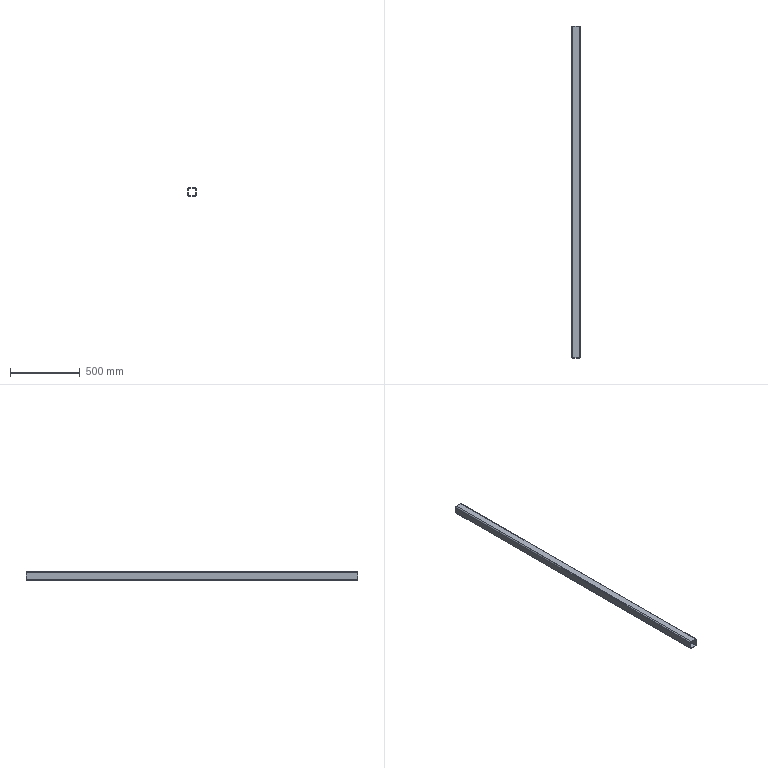Part | SolidWorks | features BaseBody 1 | 1 solid | 18 faces | box 60 x 2380 x 60 mm | volume 2034416 mm3 | plane 10 | cylinder 8 | commonest cylinder face diameters 8 x4 16 x4
STEP:
#1=CARTESIAN_POINT('',(696.,2432.,-1248.));
#2=VERTEX_POINT('',#1);
#3=CARTESIAN_POINT('',(696.,2432.,-1292.));
#4=VERTEX_POINT('',#3);
#5=CARTESIAN_POINT('',(696.,2432.,-1292.));
#6=DIRECTION('',(0.,0.,-1.));
#7=VECTOR('',#6,1000.);
#8=LINE('',#5,#7);
#9=EDGE_CURVE('',#2,#4,#8,.T.);
#10=ORIENTED_EDGE('',*,*,#9,.T.);
#11=CARTESIAN_POINT('',(696.,52.,-1292.));
#12=VERTEX_POINT('',#11);
#13=CARTESIAN_POINT('',(696.,2462.,-1292.));
#14=DIRECTION('',(0.,-1.,0.));
#15=VECTOR('',#14,1000.);
#16=LINE('',#13,#15);
#17=EDGE_CURVE('',#4,#12,#16,.T.);
#18=ORIENTED_EDGE('',*,*,#17,.T.);
#19=CARTESIAN_POINT('',(696.,52.,-1248.));
#20=VERTEX_POINT('',#19);
#21=CARTESIAN_POINT('',(696.,52.,-1292.));
#22=DIRECTION('',(0.,0.,1.));
#23=VECTOR('',#22,1000.);
#24=LINE('',#21,#23);
#25=EDGE_CURVE('',#12,#20,#24,.T.);
#26=ORIENTED_EDGE('',*,*,#25,.T.);
#27=CARTESIAN_POINT('',(696.,2462.,-1248.));
#28=DIRECTION('',(0.,1.,0.));
#29=VECTOR('',#28,1000.);
#30=LINE('',#27,#29);
#31=EDGE_CURVE('',#20,#2,#30,.T.);
#32=ORIENTED_EDGE('',*,*,#31,.T.);
#33=EDGE_LOOP('',(#10,#18,#26,#32));
#34=FACE_OUTER_BOUND('',#33,.T.);
#35=CARTESIAN_POINT('',(696.,2462.,-1292.));
#36=DIRECTION('',(-1.,0.,0.));
#37=DIRECTION('',(0.,0.,1.));
#38=AXIS2_PLACEMENT_3D('',#35,#36,#37);
#39=PLANE('',#38);
#40=ADVANCED_FACE('',(#34),#39,.T.);
#41=ORIENTED_EDGE('',*,*,#17,.F.);
#42=CARTESIAN_POINT('',(692.,2432.,-1296.));
#43=VERTEX_POINT('',#42);
#44=CARTESIAN_POINT('',(692.,2432.,-1292.));
#45=DIRECTION('',(0.,-1.,0.));
#46=DIRECTION('',(0.,0.,-1.));
#47=AXIS2_PLACEMENT_3D('',#44,#45,#46);
#48=CIRCLE('',#47,4.);
#49=EDGE_CURVE('',#43,#4,#48,.T.);
#50=ORIENTED_EDGE('',*,*,#49,.F.);
#51=CARTESIAN_POINT('',(692.,52.,-1296.));
#52=VERTEX_POINT('',#51);
#53=CARTESIAN_POINT('',(692.,2462.,-1296.));
#54=DIRECTION('',(0.,1.,0.));
#55=VECTOR('',#54,1000.);
#56=LINE('',#53,#55);
#57=EDGE_CURVE('',#52,#43,#56,.T.);
#58=ORIENTED_EDGE('',*,*,#57,.F.);
#59=CARTESIAN_POINT('',(692.,52.,-1292.));
#60=DIRECTION('',(0.,1.,0.));
#61=DIRECTION('',(0.,0.,-1.));
#62=AXIS2_PLACEMENT_3D('',#59,#60,#61);
#63=CIRCLE('',#62,4.);
#64=EDGE_CURVE('',#12,#52,#63,.T.);
#65=ORIENTED_EDGE('',*,*,#64,.F.);
#66=EDGE_LOOP('',(#41,#50,#58,#65));
#67=FACE_OUTER_BOUND('',#66,.T.);
#68=CARTESIAN_POINT('',(692.,2462.,-1292.));
#69=DIRECTION('',(0.,-1.,0.));
#70=DIRECTION('',(0.,0.,-1.));
#71=AXIS2_PLACEMENT_3D('',#68,#69,#70);
#72=CYLINDRICAL_SURFACE('',#71,4.);
#73=ADVANCED_FACE('',(#67),#72,.F.);
#74=CARTESIAN_POINT('',(692.,2432.,-1244.));
#75=VERTEX_POINT('',#74);
#76=CARTESIAN_POINT('',(692.,2432.,-1248.));
#77=DIRECTION('',(0.,-1.,0.));
#78=DIRECTION('',(0.,0.,-1.));
#79=AXIS2_PLACEMENT_3D('',#76,#77,#78);
#80=CIRCLE('',#79,4.);
#81=EDGE_CURVE('',#2,#75,#80,.T.);
#82=ORIENTED_EDGE('',*,*,#81,.T.);
#83=CARTESIAN_POINT('',(648.,2432.,-1244.));
#84=VERTEX_POINT('',#83);
#85=CARTESIAN_POINT('',(25.,2432.,-1244.));
#86=DIRECTION('',(-1.,0.,0.));
#87=VECTOR('',#86,1000.);
#88=LINE('',#85,#87);
#89=EDGE_CURVE('',#75,#84,#88,.T.);
#90=ORIENTED_EDGE('',*,*,#89,.T.);
#91=CARTESIAN_POINT('',(644.,2432.,-1248.));
#92=VERTEX_POINT('',#91);
#93=CARTESIAN_POINT('',(648.,2432.,-1248.));
#94=DIRECTION('',(0.,-1.,0.));
#95=DIRECTION('',(0.,0.,-1.));
#96=AXIS2_PLACEMENT_3D('',#93,#94,#95);
#97=CIRCLE('',#96,4.);
#98=EDGE_CURVE('',#84,#92,#97,.T.);
#99=ORIENTED_EDGE('',*,*,#98,.T.);
#100=CARTESIAN_POINT('',(644.,2432.,-1292.));
#101=VERTEX_POINT('',#100);
#102=CARTESIAN_POINT('',(644.,2432.,-1248.));
#103=DIRECTION('',(0.,0.,-1.));
#104=VECTOR('',#103,1000.);
#105=LINE('',#102,#104);
#106=EDGE_CURVE('',#92,#101,#105,.T.);
#107=ORIENTED_EDGE('',*,*,#106,.T.);
#108=CARTESIAN_POINT('',(648.,2432.,-1296.));
#109=VERTEX_POINT('',#108);
#110=CARTESIAN_POINT('',(648.,2432.,-1292.));
#111=DIRECTION('',(0.,-1.,0.));
#112=DIRECTION('',(0.,0.,-1.));
#113=AXIS2_PLACEMENT_3D('',#110,#111,#112);
#114=CIRCLE('',#113,4.);
#115=EDGE_CURVE('',#101,#109,#114,.T.);
#116=ORIENTED_EDGE('',*,*,#115,.T.);
#117=CARTESIAN_POINT('',(25.,2432.,-1296.));
#118=DIRECTION('',(1.,0.,0.));
#119=VECTOR('',#118,1000.);
#120=LINE('',#117,#119);
#121=EDGE_CURVE('',#109,#43,#120,.T.);
#122=ORIENTED_EDGE('',*,*,#121,.T.);
#123=ORIENTED_EDGE('',*,*,#49,.T.);
#124=ORIENTED_EDGE('',*,*,#9,.F.);
#125=EDGE_LOOP('',(#82,#90,#99,#107,#116,#122,#123,#124));
#126=FACE_BOUND('',#125,.T.);
#127=CARTESIAN_POINT('',(648.,2432.,-1240.));
#128=VERTEX_POINT('',#127);
#129=CARTESIAN_POINT('',(692.,2432.,-1240.));
#130=VERTEX_POINT('',#129);
#131=CARTESIAN_POINT('',(25.,2432.,-1240.));
#132=DIRECTION('',(1.,0.,0.));
#133=VECTOR('',#132,1000.);
#134=LINE('',#131,#133);
#135=EDGE_CURVE('',#128,#130,#134,.T.);
#136=ORIENTED_EDGE('',*,*,#135,.T.);
#137=CARTESIAN_POINT('',(700.,2432.,-1248.));
#138=VERTEX_POINT('',#137);
#139=CARTESIAN_POINT('',(692.,2432.,-1248.));
#140=DIRECTION('',(0.,1.,0.));
#141=DIRECTION('',(0.,0.,-1.));
#142=AXIS2_PLACEMENT_3D('',#139,#140,#141);
#143=CIRCLE('',#142,8.);
#144=EDGE_CURVE('',#130,#138,#143,.T.);
#145=ORIENTED_EDGE('',*,*,#144,.T.);
#146=CARTESIAN_POINT('',(700.,2432.,-1292.));
#147=VERTEX_POINT('',#146);
#148=CARTESIAN_POINT('',(700.,2432.,-1248.));
#149=DIRECTION('',(0.,0.,-1.));
#150=VECTOR('',#149,1000.);
#151=LINE('',#148,#150);
#152=EDGE_CURVE('',#138,#147,#151,.T.);
#153=ORIENTED_EDGE('',*,*,#152,.T.);
#154=CARTESIAN_POINT('',(692.,2432.,-1300.));
#155=VERTEX_POINT('',#154);
#156=CARTESIAN_POINT('',(692.,2432.,-1292.));
#157=DIRECTION('',(0.,1.,0.));
#158=DIRECTION('',(0.,0.,-1.));
#159=AXIS2_PLACEMENT_3D('',#156,#157,#158);
#160=CIRCLE('',#159,8.);
#161=EDGE_CURVE('',#147,#155,#160,.T.);
#162=ORIENTED_EDGE('',*,*,#161,.T.);
#163=CARTESIAN_POINT('',(648.,2432.,-1300.));
#164=VERTEX_POINT('',#163);
#165=CARTESIAN_POINT('',(25.,2432.,-1300.));
#166=DIRECTION('',(-1.,0.,0.));
#167=VECTOR('',#166,1000.);
#168=LINE('',#165,#167);
#169=EDGE_CURVE('',#155,#164,#168,.T.);
#170=ORIENTED_EDGE('',*,*,#169,.T.);
#171=CARTESIAN_POINT('',(640.,2432.,-1292.));
#172=VERTEX_POINT('',#171);
#173=CARTESIAN_POINT('',(648.,2432.,-1292.));
#174=DIRECTION('',(0.,1.,0.));
#175=DIRECTION('',(0.,0.,-1.));
#176=AXIS2_PLACEMENT_3D('',#173,#174,#175);
#177=CIRCLE('',#176,8.);
#178=EDGE_CURVE('',#164,#172,#177,.T.);
#179=ORIENTED_EDGE('',*,*,#178,.T.);
#180=CARTESIAN_POINT('',(640.,2432.,-1248.));
#181=VERTEX_POINT('',#180);
#182=CARTESIAN_POINT('',(640.,2432.,-1248.));
#183=DIRECTION('',(0.,0.,1.));
#184=VECTOR('',#183,1000.);
#185=LINE('',#182,#184);
#186=EDGE_CURVE('',#172,#181,#185,.T.);
#187=ORIENTED_EDGE('',*,*,#186,.T.);
#188=CARTESIAN_POINT('',(648.,2432.,-1248.));
#189=DIRECTION('',(0.,1.,0.));
#190=DIRECTION('',(0.,0.,-1.));
#191=AXIS2_PLACEMENT_3D('',#188,#189,#190);
#192=CIRCLE('',#191,8.);
#193=EDGE_CURVE('',#181,#128,#192,.T.);
#194=ORIENTED_EDGE('',*,*,#193,.T.);
#195=EDGE_LOOP('',(#136,#145,#153,#162,#170,#179,#187,#194));
#196=FACE_OUTER_BOUND('',#195,.T.);
#197=CARTESIAN_POINT('',(25.,2432.,-1248.));
#198=DIRECTION('',(0.,1.,0.));
#199=DIRECTION('',(0.,0.,1.));
#200=AXIS2_PLACEMENT_3D('',#197,#198,#199);
#201=PLANE('',#200);
#202=ADVANCED_FACE('',(#126,#196),#201,.T.);
#203=CARTESIAN_POINT('',(692.,52.,-1244.));
#204=VERTEX_POINT('',#203);
#205=CARTESIAN_POINT('',(692.,2462.,-1244.));
#206=DIRECTION('',(0.,-1.,0.));
#207=VECTOR('',#206,1000.);
#208=LINE('',#205,#207);
#209=EDGE_CURVE('',#75,#204,#208,.T.);
#210=ORIENTED_EDGE('',*,*,#209,.F.);
#211=ORIENTED_EDGE('',*,*,#81,.F.);
#212=ORIENTED_EDGE('',*,*,#31,.F.);
#213=CARTESIAN_POINT('',(692.,52.,-1248.));
#214=DIRECTION('',(0.,1.,0.));
#215=DIRECTION('',(0.,0.,-1.));
#216=AXIS2_PLACEMENT_3D('',#213,#214,#215);
#217=CIRCLE('',#216,4.);
#218=EDGE_CURVE('',#204,#20,#217,.T.);
#219=ORIENTED_EDGE('',*,*,#218,.F.);
#220=EDGE_LOOP('',(#210,#211,#212,#219));
#221=FACE_OUTER_BOUND('',#220,.T.);
#222=CARTESIAN_POINT('',(692.,2462.,-1248.));
#223=DIRECTION('',(0.,-1.,0.));
#224=DIRECTION('',(0.,0.,-1.));
#225=AXIS2_PLACEMENT_3D('',#222,#223,#224);
#226=CYLINDRICAL_SURFACE('',#225,4.);
#227=ADVANCED_FACE('',(#221),#226,.F.);
#228=ORIENTED_EDGE('',*,*,#218,.T.);
#229=ORIENTED_EDGE('',*,*,#25,.F.);
#230=ORIENTED_EDGE('',*,*,#64,.T.);
#231=CARTESIAN_POINT('',(648.,52.,-1296.));
#232=VERTEX_POINT('',#231);
#233=CARTESIAN_POINT('',(648.,52.,-1296.));
#234=DIRECTION('',(-1.,0.,0.));
#235=VECTOR('',#234,1000.);
#236=LINE('',#233,#235);
#237=EDGE_CURVE('',#52,#232,#236,.T.);
#238=ORIENTED_EDGE('',*,*,#237,.T.);
#239=CARTESIAN_POINT('',(644.,52.,-1292.));
#240=VERTEX_POINT('',#239);
#241=CARTESIAN_POINT('',(648.,52.,-1292.));
#242=DIRECTION('',(0.,1.,0.));
#243=DIRECTION('',(0.,0.,-1.));
#244=AXIS2_PLACEMENT_3D('',#241,#242,#243);
#245=CIRCLE('',#244,4.);
#246=EDGE_CURVE('',#232,#240,#245,.T.);
#247=ORIENTED_EDGE('',*,*,#246,.T.);
#248=CARTESIAN_POINT('',(644.,52.,-1248.));
#249=VERTEX_POINT('',#248);
#250=CARTESIAN_POINT('',(644.,52.,530.));
#251=DIRECTION('',(0.,0.,1.));
#252=VECTOR('',#251,1000.);
#253=LINE('',#250,#252);
#254=EDGE_CURVE('',#240,#249,#253,.T.);
#255=ORIENTED_EDGE('',*,*,#254,.T.);
#256=CARTESIAN_POINT('',(648.,52.,-1244.));
#257=VERTEX_POINT('',#256);
#258=CARTESIAN_POINT('',(648.,52.,-1248.));
#259=DIRECTION('',(0.,1.,0.));
#260=DIRECTION('',(0.,0.,-1.));
#261=AXIS2_PLACEMENT_3D('',#258,#259,#260);
#262=CIRCLE('',#261,4.);
#263=EDGE_CURVE('',#249,#257,#262,.T.);
#264=ORIENTED_EDGE('',*,*,#263,.T.);
#265=CARTESIAN_POINT('',(648.,52.,-1244.));
#266=DIRECTION('',(1.,0.,0.));
#267=VECTOR('',#266,1000.);
#268=LINE('',#265,#267);
#269=EDGE_CURVE('',#257,#204,#268,.T.);
#270=ORIENTED_EDGE('',*,*,#269,.T.);
#271=EDGE_LOOP('',(#228,#229,#230,#238,#247,#255,#264,#270));
#272=FACE_BOUND('',#271,.T.);
#273=CARTESIAN_POINT('',(692.,52.,-1240.));
#274=VERTEX_POINT('',#273);
#275=CARTESIAN_POINT('',(648.,52.,-1240.));
#276=VERTEX_POINT('',#275);
#277=CARTESIAN_POINT('',(648.,52.,-1240.));
#278=DIRECTION('',(-1.,0.,0.));
#279=VECTOR('',#278,1000.);
#280=LINE('',#277,#279);
#281=EDGE_CURVE('',#274,#276,#280,.T.);
#282=ORIENTED_EDGE('',*,*,#281,.T.);
#283=CARTESIAN_POINT('',(640.,52.,-1248.));
#284=VERTEX_POINT('',#283);
#285=CARTESIAN_POINT('',(648.,52.,-1248.));
#286=DIRECTION('',(0.,-1.,0.));
#287=DIRECTION('',(0.,0.,-1.));
#288=AXIS2_PLACEMENT_3D('',#285,#286,#287);
#289=CIRCLE('',#288,8.);
#290=EDGE_CURVE('',#276,#284,#289,.T.);
#291=ORIENTED_EDGE('',*,*,#290,.T.);
#292=CARTESIAN_POINT('',(640.,52.,-1292.));
#293=VERTEX_POINT('',#292);
#294=CARTESIAN_POINT('',(640.,52.,530.));
#295=DIRECTION('',(0.,0.,-1.));
#296=VECTOR('',#295,1000.);
#297=LINE('',#294,#296);
#298=EDGE_CURVE('',#284,#293,#297,.T.);
#299=ORIENTED_EDGE('',*,*,#298,.T.);
#300=CARTESIAN_POINT('',(648.,52.,-1300.));
#301=VERTEX_POINT('',#300);
#302=CARTESIAN_POINT('',(648.,52.,-1292.));
#303=DIRECTION('',(0.,-1.,0.));
#304=DIRECTION('',(0.,0.,-1.));
#305=AXIS2_PLACEMENT_3D('',#302,#303,#304);
#306=CIRCLE('',#305,8.);
#307=EDGE_CURVE('',#293,#301,#306,.T.);
#308=ORIENTED_EDGE('',*,*,#307,.T.);
#309=CARTESIAN_POINT('',(692.,52.,-1300.));
#310=VERTEX_POINT('',#309);
#311=CARTESIAN_POINT('',(648.,52.,-1300.));
#312=DIRECTION('',(1.,0.,0.));
#313=VECTOR('',#312,1000.);
#314=LINE('',#311,#313);
#315=EDGE_CURVE('',#301,#310,#314,.T.);
#316=ORIENTED_EDGE('',*,*,#315,.T.);
#317=CARTESIAN_POINT('',(700.,52.,-1292.));
#318=VERTEX_POINT('',#317);
#319=CARTESIAN_POINT('',(692.,52.,-1292.));
#320=DIRECTION('',(0.,-1.,0.));
#321=DIRECTION('',(0.,0.,-1.));
#322=AXIS2_PLACEMENT_3D('',#319,#320,#321);
#323=CIRCLE('',#322,8.);
#324=EDGE_CURVE('',#310,#318,#323,.T.);
#325=ORIENTED_EDGE('',*,*,#324,.T.);
#326=CARTESIAN_POINT('',(700.,52.,-1248.));
#327=VERTEX_POINT('',#326);
#328=CARTESIAN_POINT('',(700.,52.,530.));
#329=DIRECTION('',(0.,0.,1.));
#330=VECTOR('',#329,1000.);
#331=LINE('',#328,#330);
#332=EDGE_CURVE('',#318,#327,#331,.T.);
#333=ORIENTED_EDGE('',*,*,#332,.T.);
#334=CARTESIAN_POINT('',(692.,52.,-1248.));
#335=DIRECTION('',(0.,-1.,0.));
#336=DIRECTION('',(0.,0.,-1.));
#337=AXIS2_PLACEMENT_3D('',#334,#335,#336);
#338=CIRCLE('',#337,8.);
#339=EDGE_CURVE('',#327,#274,#338,.T.);
#340=ORIENTED_EDGE('',*,*,#339,.T.);
#341=EDGE_LOOP('',(#282,#291,#299,#308,#316,#325,#333,#340));
#342=FACE_OUTER_BOUND('',#341,.T.);
#343=CARTESIAN_POINT('',(648.,52.,530.));
#344=DIRECTION('',(0.,-1.,0.));
#345=DIRECTION('',(0.,0.,-1.));
#346=AXIS2_PLACEMENT_3D('',#343,#344,#345);
#347=PLANE('',#346);
#348=ADVANCED_FACE('',(#272,#342),#347,.T.);
#349=ORIENTED_EDGE('',*,*,#121,.F.);
#350=CARTESIAN_POINT('',(648.,2462.,-1296.));
#351=DIRECTION('',(0.,-1.,0.));
#352=VECTOR('',#351,1000.);
#353=LINE('',#350,#352);
#354=EDGE_CURVE('',#109,#232,#353,.T.);
#355=ORIENTED_EDGE('',*,*,#354,.T.);
#356=ORIENTED_EDGE('',*,*,#237,.F.);
#357=ORIENTED_EDGE('',*,*,#57,.T.);
#358=EDGE_LOOP('',(#349,#355,#356,#357));
#359=FACE_OUTER_BOUND('',#358,.T.);
#360=CARTESIAN_POINT('',(692.,2462.,-1296.));
#361=DIRECTION('',(0.,0.,1.));
#362=DIRECTION('',(1.,0.,0.));
#363=AXIS2_PLACEMENT_3D('',#360,#361,#362);
#364=PLANE('',#363);
#365=ADVANCED_FACE('',(#359),#364,.T.);
#366=ORIENTED_EDGE('',*,*,#89,.F.);
#367=ORIENTED_EDGE('',*,*,#209,.T.);
#368=ORIENTED_EDGE('',*,*,#269,.F.);
#369=CARTESIAN_POINT('',(648.,2462.,-1244.));
#370=DIRECTION('',(0.,1.,0.));
#371=VECTOR('',#370,1000.);
#372=LINE('',#369,#371);
#373=EDGE_CURVE('',#257,#84,#372,.T.);
#374=ORIENTED_EDGE('',*,*,#373,.T.);
#375=EDGE_LOOP('',(#366,#367,#368,#374));
#376=FACE_OUTER_BOUND('',#375,.T.);
#377=CARTESIAN_POINT('',(648.,2462.,-1244.));
#378=DIRECTION('',(0.,0.,-1.));
#379=DIRECTION('',(-1.,0.,0.));
#380=AXIS2_PLACEMENT_3D('',#377,#378,#379);
#381=PLANE('',#380);
#382=ADVANCED_FACE('',(#376),#381,.T.);
#383=ORIENTED_EDGE('',*,*,#354,.F.);
#384=ORIENTED_EDGE('',*,*,#115,.F.);
#385=CARTESIAN_POINT('',(644.,2462.,-1292.));
#386=DIRECTION('',(0.,1.,0.));
#387=VECTOR('',#386,1000.);
#388=LINE('',#385,#387);
#389=EDGE_CURVE('',#240,#101,#388,.T.);
#390=ORIENTED_EDGE('',*,*,#389,.F.);
#391=ORIENTED_EDGE('',*,*,#246,.F.);
#392=EDGE_LOOP('',(#383,#384,#390,#391));
#393=FACE_OUTER_BOUND('',#392,.T.);
#394=CARTESIAN_POINT('',(648.,2462.,-1292.));
#395=DIRECTION('',(0.,-1.,0.));
#396=DIRECTION('',(0.,0.,-1.));
#397=AXIS2_PLACEMENT_3D('',#394,#395,#396);
#398=CYLINDRICAL_SURFACE('',#397,4.);
#399=ADVANCED_FACE('',(#393),#398,.F.);
#400=ORIENTED_EDGE('',*,*,#106,.F.);
#401=CARTESIAN_POINT('',(644.,2462.,-1248.));
#402=DIRECTION('',(0.,-1.,0.));
#403=VECTOR('',#402,1000.);
#404=LINE('',#401,#403);
#405=EDGE_CURVE('',#92,#249,#404,.T.);
#406=ORIENTED_EDGE('',*,*,#405,.T.);
#407=ORIENTED_EDGE('',*,*,#254,.F.);
#408=ORIENTED_EDGE('',*,*,#389,.T.);
#409=EDGE_LOOP('',(#400,#406,#407,#408));
#410=FACE_OUTER_BOUND('',#409,.T.);
#411=CARTESIAN_POINT('',(644.,2462.,-1248.));
#412=DIRECTION('',(1.,0.,0.));
#413=DIRECTION('',(0.,0.,-1.));
#414=AXIS2_PLACEMENT_3D('',#411,#412,#413);
#415=PLANE('',#414);
#416=ADVANCED_FACE('',(#410),#415,.T.);
#417=ORIENTED_EDGE('',*,*,#405,.F.);
#418=ORIENTED_EDGE('',*,*,#98,.F.);
#419=ORIENTED_EDGE('',*,*,#373,.F.);
#420=ORIENTED_EDGE('',*,*,#263,.F.);
#421=EDGE_LOOP('',(#417,#418,#419,#420));
#422=FACE_OUTER_BOUND('',#421,.T.);
#423=CARTESIAN_POINT('',(648.,2462.,-1248.));
#424=DIRECTION('',(0.,-1.,0.));
#425=DIRECTION('',(0.,0.,-1.));
#426=AXIS2_PLACEMENT_3D('',#423,#424,#425);
#427=CYLINDRICAL_SURFACE('',#426,4.);
#428=ADVANCED_FACE('',(#422),#427,.F.);
#429=CARTESIAN_POINT('',(692.,2462.,-1240.));
#430=DIRECTION('',(0.,-1.,0.));
#431=VECTOR('',#430,1000.);
#432=LINE('',#429,#431);
#433=EDGE_CURVE('',#130,#274,#432,.T.);
#434=ORIENTED_EDGE('',*,*,#433,.T.);
#435=ORIENTED_EDGE('',*,*,#339,.F.);
#436=CARTESIAN_POINT('',(700.,2462.,-1248.));
#437=DIRECTION('',(0.,1.,0.));
#438=VECTOR('',#437,1000.);
#439=LINE('',#436,#438);
#440=EDGE_CURVE('',#327,#138,#439,.T.);
#441=ORIENTED_EDGE('',*,*,#440,.T.);
#442=ORIENTED_EDGE('',*,*,#144,.F.);
#443=EDGE_LOOP('',(#434,#435,#441,#442));
#444=FACE_OUTER_BOUND('',#443,.T.);
#445=CARTESIAN_POINT('',(692.,2462.,-1248.));
#446=DIRECTION('',(0.,-1.,0.));
#447=DIRECTION('',(0.,0.,-1.));
#448=AXIS2_PLACEMENT_3D('',#445,#446,#447);
#449=CYLINDRICAL_SURFACE('',#448,8.);
#450=ADVANCED_FACE('',(#444),#449,.T.);
#451=ORIENTED_EDGE('',*,*,#135,.F.);
#452=CARTESIAN_POINT('',(648.,2462.,-1240.));
#453=DIRECTION('',(0.,1.,0.));
#454=VECTOR('',#453,1000.);
#455=LINE('',#452,#454);
#456=EDGE_CURVE('',#276,#128,#455,.T.);
#457=ORIENTED_EDGE('',*,*,#456,.F.);
#458=ORIENTED_EDGE('',*,*,#281,.F.);
#459=ORIENTED_EDGE('',*,*,#433,.F.);
#460=EDGE_LOOP('',(#451,#457,#458,#459));
#461=FACE_OUTER_BOUND('',#460,.T.);
#462=CARTESIAN_POINT('',(648.,2462.,-1240.));
#463=DIRECTION('',(0.,0.,-1.));
#464=DIRECTION('',(-1.,0.,0.));
#465=AXIS2_PLACEMENT_3D('',#462,#463,#464);
#466=PLANE('',#465);
#467=ADVANCED_FACE('',(#461),#466,.F.);
#468=CARTESIAN_POINT('',(640.,2462.,-1248.));
#469=DIRECTION('',(0.,-1.,0.));
#470=VECTOR('',#469,1000.);
#471=LINE('',#468,#470);
#472=EDGE_CURVE('',#181,#284,#471,.T.);
#473=ORIENTED_EDGE('',*,*,#472,.T.);
#474=ORIENTED_EDGE('',*,*,#290,.F.);
#475=ORIENTED_EDGE('',*,*,#456,.T.);
#476=ORIENTED_EDGE('',*,*,#193,.F.);
#477=EDGE_LOOP('',(#473,#474,#475,#476));
#478=FACE_OUTER_BOUND('',#477,.T.);
#479=CARTESIAN_POINT('',(648.,2462.,-1248.));
#480=DIRECTION('',(0.,-1.,0.));
#481=DIRECTION('',(0.,0.,-1.));
#482=AXIS2_PLACEMENT_3D('',#479,#480,#481);
#483=CYLINDRICAL_SURFACE('',#482,8.);
#484=ADVANCED_FACE('',(#478),#483,.T.);
#485=ORIENTED_EDGE('',*,*,#186,.F.);
#486=CARTESIAN_POINT('',(640.,2462.,-1292.));
#487=DIRECTION('',(0.,1.,0.));
#488=VECTOR('',#487,1000.);
#489=LINE('',#486,#488);
#490=EDGE_CURVE('',#293,#172,#489,.T.);
#491=ORIENTED_EDGE('',*,*,#490,.F.);
#492=ORIENTED_EDGE('',*,*,#298,.F.);
#493=ORIENTED_EDGE('',*,*,#472,.F.);
#494=EDGE_LOOP('',(#485,#491,#492,#493));
#495=FACE_OUTER_BOUND('',#494,.T.);
#496=CARTESIAN_POINT('',(640.,2462.,-1248.));
#497=DIRECTION('',(1.,0.,0.));
#498=DIRECTION('',(0.,0.,-1.));
#499=AXIS2_PLACEMENT_3D('',#496,#497,#498);
#500=PLANE('',#499);
#501=ADVANCED_FACE('',(#495),#500,.F.);
#502=CARTESIAN_POINT('',(648.,2462.,-1300.));
#503=DIRECTION('',(0.,-1.,0.));
#504=VECTOR('',#503,1000.);
#505=LINE('',#502,#504);
#506=EDGE_CURVE('',#164,#301,#505,.T.);
#507=ORIENTED_EDGE('',*,*,#506,.T.);
#508=ORIENTED_EDGE('',*,*,#307,.F.);
#509=ORIENTED_EDGE('',*,*,#490,.T.);
#510=ORIENTED_EDGE('',*,*,#178,.F.);
#511=EDGE_LOOP('',(#507,#508,#509,#510));
#512=FACE_OUTER_BOUND('',#511,.T.);
#513=CARTESIAN_POINT('',(648.,2462.,-1292.));
#514=DIRECTION('',(0.,-1.,0.));
#515=DIRECTION('',(0.,0.,-1.));
#516=AXIS2_PLACEMENT_3D('',#513,#514,#515);
#517=CYLINDRICAL_SURFACE('',#516,8.);
#518=ADVANCED_FACE('',(#512),#517,.T.);
#519=ORIENTED_EDGE('',*,*,#169,.F.);
#520=CARTESIAN_POINT('',(692.,2462.,-1300.));
#521=DIRECTION('',(0.,1.,0.));
#522=VECTOR('',#521,1000.);
#523=LINE('',#520,#522);
#524=EDGE_CURVE('',#310,#155,#523,.T.);
#525=ORIENTED_EDGE('',*,*,#524,.F.);
#526=ORIENTED_EDGE('',*,*,#315,.F.);
#527=ORIENTED_EDGE('',*,*,#506,.F.);
#528=EDGE_LOOP('',(#519,#525,#526,#527));
#529=FACE_OUTER_BOUND('',#528,.T.);
#530=CARTESIAN_POINT('',(692.,2462.,-1300.));
#531=DIRECTION('',(0.,0.,1.));
#532=DIRECTION('',(1.,0.,0.));
#533=AXIS2_PLACEMENT_3D('',#530,#531,#532);
#534=PLANE('',#533);
#535=ADVANCED_FACE('',(#529),#534,.F.);
#536=CARTESIAN_POINT('',(700.,2462.,-1292.));
#537=DIRECTION('',(0.,-1.,0.));
#538=VECTOR('',#537,1000.);
#539=LINE('',#536,#538);
#540=EDGE_CURVE('',#147,#318,#539,.T.);
#541=ORIENTED_EDGE('',*,*,#540,.T.);
#542=ORIENTED_EDGE('',*,*,#324,.F.);
#543=ORIENTED_EDGE('',*,*,#524,.T.);
#544=ORIENTED_EDGE('',*,*,#161,.F.);
#545=EDGE_LOOP('',(#541,#542,#543,#544));
#546=FACE_OUTER_BOUND('',#545,.T.);
#547=CARTESIAN_POINT('',(692.,2462.,-1292.));
#548=DIRECTION('',(0.,-1.,0.));
#549=DIRECTION('',(0.,0.,-1.));
#550=AXIS2_PLACEMENT_3D('',#547,#548,#549);
#551=CYLINDRICAL_SURFACE('',#550,8.);
#552=ADVANCED_FACE('',(#546),#551,.T.);
#553=ORIENTED_EDGE('',*,*,#152,.F.);
#554=ORIENTED_EDGE('',*,*,#440,.F.);
#555=ORIENTED_EDGE('',*,*,#332,.F.);
#556=ORIENTED_EDGE('',*,*,#540,.F.);
#557=EDGE_LOOP('',(#553,#554,#555,#556));
#558=FACE_OUTER_BOUND('',#557,.T.);
#559=CARTESIAN_POINT('',(700.,2462.,-1292.));
#560=DIRECTION('',(-1.,0.,0.));
#561=DIRECTION('',(0.,0.,1.));
#562=AXIS2_PLACEMENT_3D('',#559,#560,#561);
#563=PLANE('',#562);
#564=ADVANCED_FACE('',(#558),#563,.F.);
#565=CLOSED_SHELL('',(#40,#73,#202,#227,#348,#365,#382,#399,#416,#428,#450,#467,#484,#501,#518,#535,#552,#564));
#566=MANIFOLD_SOLID_BREP('',#565);
#567=CARTESIAN_POINT('',(0.,0.,0.));
#568=DIRECTION('',(0.,0.,1.));
#569=DIRECTION('',(1.,0.,0.));
#570=AXIS2_PLACEMENT_3D('',#567,#568,#569);
#571=(LENGTH_UNIT()NAMED_UNIT(*)SI_UNIT(.MILLI.,.METRE.));
#572=UNCERTAINTY_MEASURE_WITH_UNIT(LENGTH_MEASURE(0.00001),#571,'','');
#573=(NAMED_UNIT(*)PLANE_ANGLE_UNIT()SI_UNIT($,.RADIAN.));
#574=(NAMED_UNIT(*)SI_UNIT($,.STERADIAN.)SOLID_ANGLE_UNIT());
#575=(GEOMETRIC_REPRESENTATION_CONTEXT(3)GLOBAL_UNCERTAINTY_ASSIGNED_CONTEXT((#572))GLOBAL_UNIT_ASSIGNED_CONTEXT((#571,#573,#574))REPRESENTATION_CONTEXT('',''));
#576=ADVANCED_BREP_SHAPE_REPRESENTATION('',(#566,#570),#575);